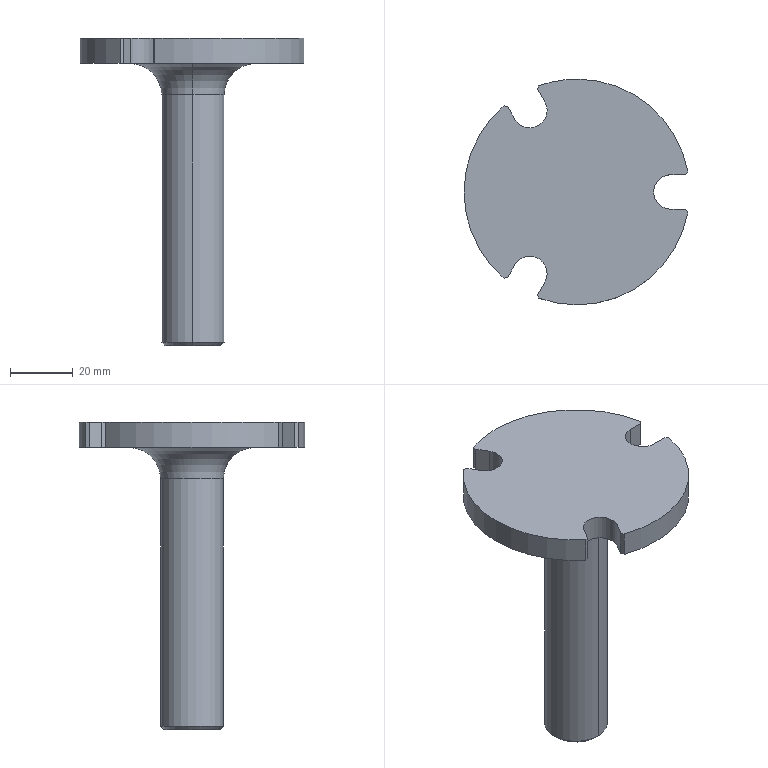NC program | NX | posted with a generic post | part box 71.434 x 72 x 98 mm
Lines 10922 to 11060 of 11060:
(ZLEVEL_PROFILE_COPY , TOOL : D6JING)
N21842 T08 M6
N21844 G54
N21846 G17 G0 G90 X-14.881 Y-38.821 S7500 M3
N21848 G43 Z30. H8
N21850 Z-7.5
N21852 G94 G1 Z-9. F1000.
N21854 X-14.199 Y-38.138
N21856 G3 X-14.044 Y-37.558 R0.6
N21858 G1 X-14.985 Y-34.053
N21860 X-15.14 Y-33.471
N21862 G2 X-14.707 Y-30.984 R3.
N21864 G1 X-14.709 Y-30.97
N21866 X-14.618 Y-30.811
N21868 X-14.613 Y-30.8
N21870 X-12.552 Y-27.231
N21872 G3 X-13.467 Y-23.816 R2.5
N21874 X-16.882 Y-24.731 R2.5
N21876 G1 X-18.939 Y-28.294
N21878 X-18.95 Y-28.306
N21880 X-19.025 Y-28.435
N21882 X-19.029 Y-28.447
N21884 X-19.04 Y-28.442
N21886 G2 X-20.993 Y-30.093 R3.
N21888 G1 X-21.565 Y-30.246
N21890 X-25.351 Y-31.258
N21892 G3 X-25.776 Y-31.682 R0.6
N21894 G1 X-26.011 Y-32.559
N21896 Z-7.5
N21898 G0 Z30.
N21900 X41.584 Y6.42
N21902 Z-7.5
N21904 G1 Z-9.
N21906 X40.686 Y6.661
N21908 G3 X40.107 Y6.505 R0.6
N21910 G1 X37.838 Y4.236
N21912 X37.313 Y3.71
N21914 X37.184 Y3.586
N21916 X37.166 Y3.581
N21918 G2 X34.86 Y2.5 R3.
N21920 G1 X30.283
N21922 G3 X27.783 Y0. R2.5
N21924 X30.283 Y-2.5 R2.5
N21926 G1 X34.86
N21928 G2 X36.982 Y-3.379 R3.
N21930 G1 X37.465 Y-3.862
N21932 X40.107 Y-6.505
N21934 G3 X40.687 Y-6.66 R0.6
N21936 G1 X41.585 Y-6.419
N21938 Z-7.5
N21940 G0 Z30.
N21942 X-26.01 Y32.56
N21944 Z-7.5
N21946 G1 Z-9.
N21948 X-25.776 Y31.684
N21950 G3 X-25.351 Y31.26 R0.6
N21952 G1 X-22.149 Y30.402
N21954 X-20.993 Y30.093
N21956 G2 X-19.171 Y28.695 R3.
N21958 G1 X-16.882 Y24.731
N21960 G3 X-13.467 Y23.816 R2.5
N21962 X-12.552 Y27.231 R2.5
N21964 G1 X-14.841 Y31.195
N21966 G2 X-15.06 Y33.725 R3.
N21968 G1 X-15.066 Y33.723
N21970 X-15.069 Y33.728
N21972 X-15.067 Y33.732
N21974 X-15.023 Y33.901
N21976 X-15.022 Y33.912
N21978 X-14.832 Y34.623
N21980 X-14.755 Y34.872
N21982 X-14.761 Y34.886
N21984 X-14.044 Y37.558
N21986 G3 X-14.199 Y38.138 R0.6
N21988 G1 X-14.881 Y38.821
N21990 Z-7.5
N21992 G0 Z30.
N21994 M5
(PLANAR_MILL_COPY , TOOL : D6A45)
N21996 T07 M6
N21998 G54
N22000 G17 G0 G90 X-23.623 Y29.866 S7500 M3
N22002 G43 Z30. H7
N22004 Z0.5
N22006 G94 G1 Z-1. F1250.
N22008 X-23.414 Y29.085
N22010 G3 X-22.707 Y28.378 R1.
N22012 G1 X-21.576 Y28.075
N22014 G2 X-20.969 Y27.609 R1.
N22016 G1 X-18.701 Y23.681
N22018 G3 X-12.417 Y21.997 R4.6
N22020 X-10.733 Y28.281 R4.6
N22022 G1 X-13.001 Y32.209
N22024 G2 X-13.101 Y32.968 R1.
N22026 G1 X-12.798 Y34.098
N22028 G3 X-13.057 Y35.064 R1.
N22030 G1 X-13.629 Y35.636
N22032 Z0.5
N22034 G0 Z30.
N22036 X38.1 Y5.77
N22038 Z0.5
N22040 G1 Z-1.
N22042 X37.319 Y5.979
N22044 G3 X36.354 Y5.721 R1.
N22046 G1 X35.526 Y4.893
N22048 G2 X34.819 Y4.6 R1.
N22050 G1 X30.283
N22052 G3 X25.683 Y0. R4.6
N22054 X30.283 Y-4.6 R4.6
N22056 G1 X34.819
N22058 G2 X35.526 Y-4.893 R1.
N22060 G1 X36.354 Y-5.721
N22062 G3 X37.319 Y-5.979 R1.
N22064 G1 X38.1 Y-5.77
N22066 Z0.5
N22068 G0 Z30.
N22070 X-13.629 Y-35.636
N22072 Z0.5
N22074 G1 Z-1.
N22076 X-13.057 Y-35.064
N22078 G3 X-12.798 Y-34.098 R1.
N22080 G1 X-13.101 Y-32.968
N22082 G2 X-13.001 Y-32.209 R1.
N22084 G1 X-10.733 Y-28.281
N22086 G3 X-12.417 Y-21.997 R4.6
N22088 X-18.701 Y-23.681 R4.6
N22090 G1 X-20.969 Y-27.609
N22092 G2 X-21.576 Y-28.075 R1.
N22094 G1 X-22.707 Y-28.378
N22096 G3 X-23.414 Y-29.085 R1.
N22098 G1 X-23.623 Y-29.866
N22100 Z0.5
N22102 G0 Z30.
N22104 M5
N22106 M2